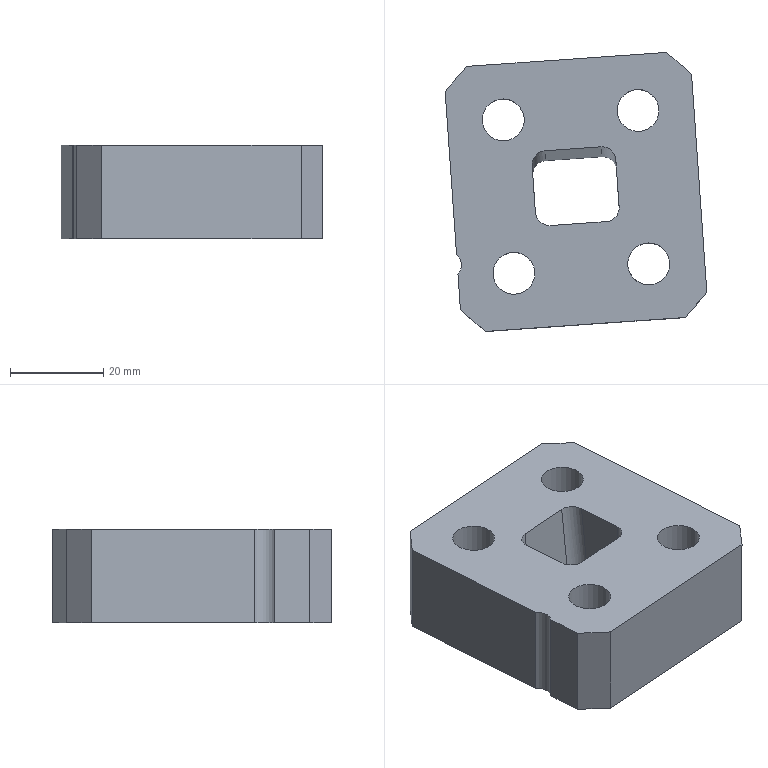Part | STEP file | 车灯-后视镜_id94_x_t | 1 solid | 32 faces | box 56.149 x 59.861 x 20 mm | volume 45570 mm3 | plane 19 | cylinder 13 | commonest cylinder face diameters 6 x5 9 x4 14 x4
STEP:
#1=CARTESIAN_POINT('',(-19.757,-26.993,-160.5));
#2=VERTEX_POINT('',#1);
#3=CARTESIAN_POINT('',(-19.757,-26.993,-140.5));
#4=VERTEX_POINT('',#3);
#5=CARTESIAN_POINT('',(-19.757,-26.993,60.));
#6=DIRECTION('',(0.,0.,1.));
#7=VECTOR('',#6,1.);
#8=LINE('',#5,#7);
#9=EDGE_CURVE('',#2,#4,#8,.T.);
#10=ORIENTED_EDGE('',*,*,#9,.F.);
#11=CARTESIAN_POINT('',(-19.225,-34.604,-160.5));
#12=VERTEX_POINT('',#11);
#13=CARTESIAN_POINT('',(-19.643,-28.63,-160.5));
#14=DIRECTION('',(-0.06976,0.9976,0.));
#15=VECTOR('',#14,1.);
#16=LINE('',#13,#15);
#17=EDGE_CURVE('',#12,#2,#16,.T.);
#18=ORIENTED_EDGE('',*,*,#17,.F.);
#19=CARTESIAN_POINT('',(-19.225,-34.604,-140.5));
#20=VERTEX_POINT('',#19);
#21=CARTESIAN_POINT('',(-19.225,-34.604,-144.5));
#22=DIRECTION('',(0.,0.,-1.));
#23=VECTOR('',#22,1.);
#24=LINE('',#21,#23);
#25=EDGE_CURVE('',#20,#12,#24,.T.);
#26=ORIENTED_EDGE('',*,*,#25,.F.);
#27=CARTESIAN_POINT('',(-19.643,-28.63,-140.5));
#28=DIRECTION('',(0.06976,-0.9976,0.));
#29=VECTOR('',#28,1.);
#30=LINE('',#27,#29);
#31=EDGE_CURVE('',#4,#20,#30,.T.);
#32=ORIENTED_EDGE('',*,*,#31,.F.);
#33=EDGE_LOOP('',(#10,#18,#26,#32));
#34=FACE_OUTER_BOUND('',#33,.T.);
#35=CARTESIAN_POINT('',(-19.643,-28.63,-138.5));
#36=DIRECTION('',(-0.9976,-0.06976,0.));
#37=DIRECTION('',(0.,0.,-1.));
#38=AXIS2_PLACEMENT_3D('',#35,#36,#37);
#39=PLANE('',#38);
#40=ADVANCED_FACE('',(#34),#39,.T.);
#41=CARTESIAN_POINT('',(-20.056,-22.715,-160.5));
#42=VERTEX_POINT('',#41);
#43=CARTESIAN_POINT('',(-22.,-25.,-160.5));
#44=DIRECTION('',(0.,0.,-1.));
#45=DIRECTION('',(0.,1.,0.));
#46=AXIS2_PLACEMENT_3D('',#43,#44,#45);
#47=CIRCLE('',#46,3.);
#48=EDGE_CURVE('',#42,#2,#47,.T.);
#49=ORIENTED_EDGE('',*,*,#48,.F.);
#50=CARTESIAN_POINT('',(-22.504,12.282,-160.5));
#51=VERTEX_POINT('',#50);
#52=CARTESIAN_POINT('',(-19.643,-28.63,-160.5));
#53=DIRECTION('',(-0.06976,0.9976,0.));
#54=VECTOR('',#53,1.);
#55=LINE('',#52,#54);
#56=EDGE_CURVE('',#42,#51,#55,.T.);
#57=ORIENTED_EDGE('',*,*,#56,.T.);
#58=CARTESIAN_POINT('',(-17.865,17.618,-160.5));
#59=VERTEX_POINT('',#58);
#60=CARTESIAN_POINT('',(-22.504,12.282,-160.5));
#61=DIRECTION('',(-0.6561,-0.7547,0.));
#62=VECTOR('',#61,1.);
#63=LINE('',#60,#62);
#64=EDGE_CURVE('',#59,#51,#63,.T.);
#65=ORIENTED_EDGE('',*,*,#64,.F.);
#66=CARTESIAN_POINT('',(25.031,20.618,-160.5));
#67=VERTEX_POINT('',#66);
#68=CARTESIAN_POINT('',(2.662,19.054,-160.5));
#69=DIRECTION('',(0.9976,0.06976,0.));
#70=VECTOR('',#69,1.);
#71=LINE('',#68,#70);
#72=EDGE_CURVE('',#59,#67,#71,.T.);
#73=ORIENTED_EDGE('',*,*,#72,.T.);
#74=CARTESIAN_POINT('',(30.367,15.979,-160.5));
#75=VERTEX_POINT('',#74);
#76=CARTESIAN_POINT('',(25.031,20.618,-160.5));
#77=DIRECTION('',(-0.7547,0.6561,0.));
#78=VECTOR('',#77,1.);
#79=LINE('',#76,#78);
#80=EDGE_CURVE('',#75,#67,#79,.T.);
#81=ORIENTED_EDGE('',*,*,#80,.F.);
#82=CARTESIAN_POINT('',(33.646,-30.907,-160.5));
#83=VERTEX_POINT('',#82);
#84=CARTESIAN_POINT('',(33.228,-24.933,-160.5));
#85=DIRECTION('',(0.06976,-0.9976,0.));
#86=VECTOR('',#85,1.);
#87=LINE('',#84,#86);
#88=EDGE_CURVE('',#75,#83,#87,.T.);
#89=ORIENTED_EDGE('',*,*,#88,.T.);
#90=CARTESIAN_POINT('',(29.007,-36.243,-160.5));
#91=VERTEX_POINT('',#90);
#92=CARTESIAN_POINT('',(29.007,-36.243,-160.5));
#93=DIRECTION('',(0.6561,0.7547,0.));
#94=VECTOR('',#93,1.);
#95=LINE('',#92,#94);
#96=EDGE_CURVE('',#91,#83,#95,.T.);
#97=ORIENTED_EDGE('',*,*,#96,.F.);
#98=CARTESIAN_POINT('',(-13.889,-39.243,-160.5));
#99=VERTEX_POINT('',#98);
#100=CARTESIAN_POINT('',(6.639,-37.808,-160.5));
#101=DIRECTION('',(-0.9976,-0.06976,0.));
#102=VECTOR('',#101,1.);
#103=LINE('',#100,#102);
#104=EDGE_CURVE('',#91,#99,#103,.T.);
#105=ORIENTED_EDGE('',*,*,#104,.T.);
#106=CARTESIAN_POINT('',(-13.889,-39.243,-160.5));
#107=DIRECTION('',(0.7547,-0.6561,0.));
#108=VECTOR('',#107,1.);
#109=LINE('',#106,#108);
#110=EDGE_CURVE('',#12,#99,#109,.T.);
#111=ORIENTED_EDGE('',*,*,#110,.F.);
#112=ORIENTED_EDGE('',*,*,#17,.T.);
#113=EDGE_LOOP('',(#49,#57,#65,#73,#81,#89,#97,#105,#111,#112));
#114=FACE_BOUND('',#113,.T.);
#115=CARTESIAN_POINT('',(-9.984,-0.864,-160.5));
#116=VERTEX_POINT('',#115);
#117=CARTESIAN_POINT('',(-10.045,6.136,-160.5));
#118=DIRECTION('',(0.,0.,1.));
#119=DIRECTION('',(0.008727,-1.,0.));
#120=AXIS2_PLACEMENT_3D('',#117,#118,#119);
#121=CIRCLE('',#120,7.);
#122=EDGE_CURVE('',#116,#116,#121,.T.);
#123=ORIENTED_EDGE('',*,*,#122,.T.);
#124=EDGE_LOOP('',(#123));
#125=FACE_BOUND('',#124,.T.);
#126=CARTESIAN_POINT('',(-7.743,-19.784,-160.5));
#127=VERTEX_POINT('',#126);
#128=CARTESIAN_POINT('',(-7.743,-26.784,-160.5));
#129=DIRECTION('',(0.,0.,-1.));
#130=DIRECTION('',(0.,1.,0.));
#131=AXIS2_PLACEMENT_3D('',#128,#129,#130);
#132=CIRCLE('',#131,7.);
#133=EDGE_CURVE('',#127,#127,#132,.T.);
#134=ORIENTED_EDGE('',*,*,#133,.F.);
#135=EDGE_LOOP('',(#134));
#136=FACE_BOUND('',#135,.T.);
#137=CARTESIAN_POINT('',(18.885,15.159,-160.5));
#138=VERTEX_POINT('',#137);
#139=CARTESIAN_POINT('',(18.885,8.159,-160.5));
#140=DIRECTION('',(0.,0.,-1.));
#141=DIRECTION('',(0.,1.,0.));
#142=AXIS2_PLACEMENT_3D('',#139,#140,#141);
#143=CIRCLE('',#142,7.);
#144=EDGE_CURVE('',#138,#138,#143,.T.);
#145=ORIENTED_EDGE('',*,*,#144,.F.);
#146=EDGE_LOOP('',(#145));
#147=FACE_BOUND('',#146,.T.);
#148=CARTESIAN_POINT('',(21.187,-17.761,-160.5));
#149=VERTEX_POINT('',#148);
#150=CARTESIAN_POINT('',(21.187,-24.761,-160.5));
#151=DIRECTION('',(0.,0.,1.));
#152=DIRECTION('',(0.,1.,0.));
#153=AXIS2_PLACEMENT_3D('',#150,#151,#152);
#154=CIRCLE('',#153,7.);
#155=EDGE_CURVE('',#149,#149,#154,.T.);
#156=ORIENTED_EDGE('',*,*,#155,.T.);
#157=EDGE_LOOP('',(#156));
#158=FACE_BOUND('',#157,.T.);
#159=CARTESIAN_POINT('',(-3.697,-5.793,-160.5));
#160=VERTEX_POINT('',#159);
#161=CARTESIAN_POINT('',(-0.9148,-2.575,-160.5));
#162=VERTEX_POINT('',#161);
#163=CARTESIAN_POINT('',(-0.7043,-5.584,-160.5));
#164=DIRECTION('',(0.,0.,-1.));
#165=DIRECTION('',(-0.06976,0.9976,0.));
#166=AXIS2_PLACEMENT_3D('',#163,#164,#165);
#167=ELLIPSE('',#166,3.017,3.);
#168=EDGE_CURVE('',#160,#162,#167,.T.);
#169=ORIENTED_EDGE('',*,*,#168,.F.);
#170=CARTESIAN_POINT('',(-2.996,-15.824,-160.5));
#171=VERTEX_POINT('',#170);
#172=CARTESIAN_POINT('',(-2.185,-27.409,-160.5));
#173=DIRECTION('',(0.06976,-0.9976,0.));
#174=VECTOR('',#173,1.);
#175=LINE('',#172,#174);
#176=EDGE_CURVE('',#160,#171,#175,.T.);
#177=ORIENTED_EDGE('',*,*,#176,.T.);
#178=CARTESIAN_POINT('',(0.2075,-18.624,-160.5));
#179=VERTEX_POINT('',#178);
#180=CARTESIAN_POINT('',(-0.002931,-15.614,-160.5));
#181=DIRECTION('',(0.,0.,-1.));
#182=DIRECTION('',(-0.06976,0.9976,0.));
#183=AXIS2_PLACEMENT_3D('',#180,#181,#182);
#184=ELLIPSE('',#183,3.017,3.);
#185=EDGE_CURVE('',#179,#171,#184,.T.);
#186=ORIENTED_EDGE('',*,*,#185,.F.);
#187=CARTESIAN_POINT('',(12.178,-17.786,-160.5));
#188=VERTEX_POINT('',#187);
#189=CARTESIAN_POINT('',(5.272,-18.269,-160.5));
#190=DIRECTION('',(-0.9976,-0.06976,0.));
#191=VECTOR('',#190,1.);
#192=LINE('',#189,#191);
#193=EDGE_CURVE('',#188,#179,#192,.T.);
#194=ORIENTED_EDGE('',*,*,#193,.F.);
#195=CARTESIAN_POINT('',(14.961,-14.568,-160.5));
#196=VERTEX_POINT('',#195);
#197=CARTESIAN_POINT('',(11.968,-14.777,-160.5));
#198=DIRECTION('',(0.,0.,-1.));
#199=DIRECTION('',(0.06976,-0.9976,0.));
#200=AXIS2_PLACEMENT_3D('',#197,#198,#199);
#201=ELLIPSE('',#200,3.017,3.);
#202=EDGE_CURVE('',#196,#188,#201,.T.);
#203=ORIENTED_EDGE('',*,*,#202,.F.);
#204=CARTESIAN_POINT('',(14.259,-4.537,-160.5));
#205=VERTEX_POINT('',#204);
#206=CARTESIAN_POINT('',(15.771,-26.154,-160.5));
#207=DIRECTION('',(0.06976,-0.9976,0.));
#208=VECTOR('',#207,1.);
#209=LINE('',#206,#208);
#210=EDGE_CURVE('',#205,#196,#209,.T.);
#211=ORIENTED_EDGE('',*,*,#210,.F.);
#212=CARTESIAN_POINT('',(11.056,-1.738,-160.5));
#213=VERTEX_POINT('',#212);
#214=CARTESIAN_POINT('',(11.266,-4.747,-160.5));
#215=DIRECTION('',(0.,0.,-1.));
#216=DIRECTION('',(-0.06976,0.9976,0.));
#217=AXIS2_PLACEMENT_3D('',#214,#215,#216);
#218=ELLIPSE('',#217,3.017,3.);
#219=EDGE_CURVE('',#213,#205,#218,.T.);
#220=ORIENTED_EDGE('',*,*,#219,.F.);
#221=CARTESIAN_POINT('',(4.15,-2.22,-160.5));
#222=DIRECTION('',(0.9976,0.06976,0.));
#223=VECTOR('',#222,1.);
#224=LINE('',#221,#223);
#225=EDGE_CURVE('',#162,#213,#224,.T.);
#226=ORIENTED_EDGE('',*,*,#225,.F.);
#227=EDGE_LOOP('',(#169,#177,#186,#194,#203,#211,#220,#226));
#228=FACE_BOUND('',#227,.T.);
#229=CARTESIAN_POINT('',(5.872,-26.846,-160.5));
#230=DIRECTION('',(0.,0.,-1.));
#231=DIRECTION('',(-0.06976,0.9976,0.));
#232=AXIS2_PLACEMENT_3D('',#229,#230,#231);
#233=PLANE('',#232);
#234=ADVANCED_FACE('',(#114,#125,#136,#147,#158,#228),#233,.T.);
#235=CARTESIAN_POINT('',(-20.056,-22.715,-140.5));
#236=VERTEX_POINT('',#235);
#237=CARTESIAN_POINT('',(-22.,-25.,-140.5));
#238=DIRECTION('',(0.,0.,1.));
#239=DIRECTION('',(0.,-1.,0.));
#240=AXIS2_PLACEMENT_3D('',#237,#238,#239);
#241=CIRCLE('',#240,3.);
#242=EDGE_CURVE('',#4,#236,#241,.T.);
#243=ORIENTED_EDGE('',*,*,#242,.F.);
#244=ORIENTED_EDGE('',*,*,#31,.T.);
#245=CARTESIAN_POINT('',(-13.889,-39.243,-140.5));
#246=VERTEX_POINT('',#245);
#247=CARTESIAN_POINT('',(-13.889,-39.243,-140.5));
#248=DIRECTION('',(-0.7547,0.6561,0.));
#249=VECTOR('',#248,1.);
#250=LINE('',#247,#249);
#251=EDGE_CURVE('',#246,#20,#250,.T.);
#252=ORIENTED_EDGE('',*,*,#251,.F.);
#253=CARTESIAN_POINT('',(29.007,-36.243,-140.5));
#254=VERTEX_POINT('',#253);
#255=CARTESIAN_POINT('',(6.639,-37.808,-140.5));
#256=DIRECTION('',(0.9976,0.06976,0.));
#257=VECTOR('',#256,1.);
#258=LINE('',#255,#257);
#259=EDGE_CURVE('',#246,#254,#258,.T.);
#260=ORIENTED_EDGE('',*,*,#259,.T.);
#261=CARTESIAN_POINT('',(33.646,-30.907,-140.5));
#262=VERTEX_POINT('',#261);
#263=CARTESIAN_POINT('',(29.007,-36.243,-140.5));
#264=DIRECTION('',(-0.6561,-0.7547,0.));
#265=VECTOR('',#264,1.);
#266=LINE('',#263,#265);
#267=EDGE_CURVE('',#262,#254,#266,.T.);
#268=ORIENTED_EDGE('',*,*,#267,.F.);
#269=CARTESIAN_POINT('',(30.367,15.979,-140.5));
#270=VERTEX_POINT('',#269);
#271=CARTESIAN_POINT('',(33.228,-24.933,-140.5));
#272=DIRECTION('',(-0.06976,0.9976,0.));
#273=VECTOR('',#272,1.);
#274=LINE('',#271,#273);
#275=EDGE_CURVE('',#262,#270,#274,.T.);
#276=ORIENTED_EDGE('',*,*,#275,.T.);
#277=CARTESIAN_POINT('',(25.031,20.618,-140.5));
#278=VERTEX_POINT('',#277);
#279=CARTESIAN_POINT('',(25.031,20.618,-140.5));
#280=DIRECTION('',(0.7547,-0.6561,0.));
#281=VECTOR('',#280,1.);
#282=LINE('',#279,#281);
#283=EDGE_CURVE('',#278,#270,#282,.T.);
#284=ORIENTED_EDGE('',*,*,#283,.F.);
#285=CARTESIAN_POINT('',(-17.865,17.618,-140.5));
#286=VERTEX_POINT('',#285);
#287=CARTESIAN_POINT('',(2.662,19.054,-140.5));
#288=DIRECTION('',(-0.9976,-0.06976,0.));
#289=VECTOR('',#288,1.);
#290=LINE('',#287,#289);
#291=EDGE_CURVE('',#278,#286,#290,.T.);
#292=ORIENTED_EDGE('',*,*,#291,.T.);
#293=CARTESIAN_POINT('',(-22.504,12.282,-140.5));
#294=VERTEX_POINT('',#293);
#295=CARTESIAN_POINT('',(-22.504,12.282,-140.5));
#296=DIRECTION('',(0.6561,0.7547,0.));
#297=VECTOR('',#296,1.);
#298=LINE('',#295,#297);
#299=EDGE_CURVE('',#294,#286,#298,.T.);
#300=ORIENTED_EDGE('',*,*,#299,.F.);
#301=CARTESIAN_POINT('',(-19.643,-28.63,-140.5));
#302=DIRECTION('',(0.06976,-0.9976,0.));
#303=VECTOR('',#302,1.);
#304=LINE('',#301,#303);
#305=EDGE_CURVE('',#294,#236,#304,.T.);
#306=ORIENTED_EDGE('',*,*,#305,.T.);
#307=EDGE_LOOP('',(#243,#244,#252,#260,#268,#276,#284,#292,#300,#306));
#308=FACE_BOUND('',#307,.T.);
#309=CARTESIAN_POINT('',(-10.084,10.636,-140.5));
#310=VERTEX_POINT('',#309);
#311=CARTESIAN_POINT('',(-10.045,6.136,-140.5));
#312=DIRECTION('',(0.,0.,-1.));
#313=DIRECTION('',(-0.008727,1.,0.));
#314=AXIS2_PLACEMENT_3D('',#311,#312,#313);
#315=CIRCLE('',#314,4.5);
#316=EDGE_CURVE('',#310,#310,#315,.T.);
#317=ORIENTED_EDGE('',*,*,#316,.T.);
#318=EDGE_LOOP('',(#317));
#319=FACE_BOUND('',#318,.T.);
#320=CARTESIAN_POINT('',(-7.743,-31.284,-140.5));
#321=VERTEX_POINT('',#320);
#322=CARTESIAN_POINT('',(-7.743,-26.784,-140.5));
#323=DIRECTION('',(0.,0.,1.));
#324=DIRECTION('',(0.,-1.,0.));
#325=AXIS2_PLACEMENT_3D('',#322,#323,#324);
#326=CIRCLE('',#325,4.5);
#327=EDGE_CURVE('',#321,#321,#326,.T.);
#328=ORIENTED_EDGE('',*,*,#327,.F.);
#329=EDGE_LOOP('',(#328));
#330=FACE_BOUND('',#329,.T.);
#331=CARTESIAN_POINT('',(18.885,3.659,-140.5));
#332=VERTEX_POINT('',#331);
#333=CARTESIAN_POINT('',(18.885,8.159,-140.5));
#334=DIRECTION('',(0.,0.,1.));
#335=DIRECTION('',(0.,-1.,0.));
#336=AXIS2_PLACEMENT_3D('',#333,#334,#335);
#337=CIRCLE('',#336,4.5);
#338=EDGE_CURVE('',#332,#332,#337,.T.);
#339=ORIENTED_EDGE('',*,*,#338,.F.);
#340=EDGE_LOOP('',(#339));
#341=FACE_BOUND('',#340,.T.);
#342=CARTESIAN_POINT('',(21.187,-29.261,-140.5));
#343=VERTEX_POINT('',#342);
#344=CARTESIAN_POINT('',(21.187,-24.761,-140.5));
#345=DIRECTION('',(0.,0.,-1.));
#346=DIRECTION('',(0.,-1.,0.));
#347=AXIS2_PLACEMENT_3D('',#344,#345,#346);
#348=CIRCLE('',#347,4.5);
#349=EDGE_CURVE('',#343,#343,#348,.T.);
#350=ORIENTED_EDGE('',*,*,#349,.T.);
#351=EDGE_LOOP('',(#350));
#352=FACE_BOUND('',#351,.T.);
#353=CARTESIAN_POINT('',(-3.142,-13.727,-140.5));
#354=VERTEX_POINT('',#353);
#355=CARTESIAN_POINT('',(0.06086,-16.527,-140.5));
#356=VERTEX_POINT('',#355);
#357=CARTESIAN_POINT('',(-0.1496,-13.517,-140.5));
#358=DIRECTION('',(0.,0.,1.));
#359=DIRECTION('',(-0.06976,0.9976,0.));
#360=AXIS2_PLACEMENT_3D('',#357,#358,#359);
#361=ELLIPSE('',#360,3.017,3.);
#362=EDGE_CURVE('',#354,#356,#361,.T.);
#363=ORIENTED_EDGE('',*,*,#362,.F.);
#364=CARTESIAN_POINT('',(-3.844,-3.696,-140.5));
#365=VERTEX_POINT('',#364);
#366=CARTESIAN_POINT('',(-2.185,-27.409,-140.5));
#367=DIRECTION('',(-0.06976,0.9976,0.));
#368=VECTOR('',#367,1.);
#369=LINE('',#366,#368);
#370=EDGE_CURVE('',#354,#365,#369,.T.);
#371=ORIENTED_EDGE('',*,*,#370,.T.);
#372=CARTESIAN_POINT('',(-1.061,-0.4776,-140.5));
#373=VERTEX_POINT('',#372);
#374=CARTESIAN_POINT('',(-0.851,-3.487,-140.5));
#375=DIRECTION('',(0.,0.,1.));
#376=DIRECTION('',(-0.06976,0.9976,0.));
#377=AXIS2_PLACEMENT_3D('',#374,#375,#376);
#378=ELLIPSE('',#377,3.017,3.);
#379=EDGE_CURVE('',#373,#365,#378,.T.);
#380=ORIENTED_EDGE('',*,*,#379,.F.);
#381=CARTESIAN_POINT('',(10.909,0.3594,-140.5));
#382=VERTEX_POINT('',#381);
#383=CARTESIAN_POINT('',(4.003,-0.1235,-140.5));
#384=DIRECTION('',(-0.9976,-0.06976,0.));
#385=VECTOR('',#384,1.);
#386=LINE('',#383,#385);
#387=EDGE_CURVE('',#382,#373,#386,.T.);
#388=ORIENTED_EDGE('',*,*,#387,.F.);
#389=CARTESIAN_POINT('',(14.112,-2.44,-140.5));
#390=VERTEX_POINT('',#389);
#391=CARTESIAN_POINT('',(11.12,-2.65,-140.5));
#392=DIRECTION('',(0.,0.,1.));
#393=DIRECTION('',(-0.06976,0.9976,0.));
#394=AXIS2_PLACEMENT_3D('',#391,#392,#393);
#395=ELLIPSE('',#394,3.017,3.);
#396=EDGE_CURVE('',#390,#382,#395,.T.);
#397=ORIENTED_EDGE('',*,*,#396,.F.);
#398=CARTESIAN_POINT('',(14.814,-12.471,-140.5));
#399=VERTEX_POINT('',#398);
#400=CARTESIAN_POINT('',(15.771,-26.154,-140.5));
#401=DIRECTION('',(-0.06976,0.9976,0.));
#402=VECTOR('',#401,1.);
#403=LINE('',#400,#402);
#404=EDGE_CURVE('',#399,#390,#403,.T.);
#405=ORIENTED_EDGE('',*,*,#404,.F.);
#406=CARTESIAN_POINT('',(12.032,-15.689,-140.5));
#407=VERTEX_POINT('',#406);
#408=CARTESIAN_POINT('',(11.821,-12.68,-140.5));
#409=DIRECTION('',(0.,0.,1.));
#410=DIRECTION('',(0.06976,-0.9976,0.));
#411=AXIS2_PLACEMENT_3D('',#408,#409,#410);
#412=ELLIPSE('',#411,3.017,3.);
#413=EDGE_CURVE('',#407,#399,#412,.T.);
#414=ORIENTED_EDGE('',*,*,#413,.F.);
#415=CARTESIAN_POINT('',(5.126,-16.172,-140.5));
#416=DIRECTION('',(0.9976,0.06976,0.));
#417=VECTOR('',#416,1.);
#418=LINE('',#415,#417);
#419=EDGE_CURVE('',#356,#407,#418,.T.);
#420=ORIENTED_EDGE('',*,*,#419,.F.);
#421=EDGE_LOOP('',(#363,#371,#380,#388,#397,#405,#414,#420));
#422=FACE_BOUND('',#421,.T.);
#423=CARTESIAN_POINT('',(5.872,-26.846,-140.5));
#424=DIRECTION('',(0.,0.,1.));
#425=DIRECTION('',(0.06976,-0.9976,0.));
#426=AXIS2_PLACEMENT_3D('',#423,#424,#425);
#427=PLANE('',#426);
#428=ADVANCED_FACE('',(#308,#319,#330,#341,#352,#422),#427,.T.);
#429=ORIENTED_EDGE('',*,*,#275,.F.);
#430=CARTESIAN_POINT('',(33.646,-30.907,-144.5));
#431=DIRECTION('',(0.,0.,1.));
#432=VECTOR('',#431,1.);
#433=LINE('',#430,#432);
#434=EDGE_CURVE('',#83,#262,#433,.T.);
#435=ORIENTED_EDGE('',*,*,#434,.F.);
#436=ORIENTED_EDGE('',*,*,#88,.F.);
#437=CARTESIAN_POINT('',(30.367,15.979,-138.5));
#438=DIRECTION('',(0.,0.,-1.));
#439=VECTOR('',#438,1.);
#440=LINE('',#437,#439);
#441=EDGE_CURVE('',#270,#75,#440,.T.);
#442=ORIENTED_EDGE('',*,*,#441,.F.);
#443=EDGE_LOOP('',(#429,#435,#436,#442));
#444=FACE_OUTER_BOUND('',#443,.T.);
#445=CARTESIAN_POINT('',(33.228,-24.933,-138.5));
#446=DIRECTION('',(0.9976,0.06976,0.));
#447=DIRECTION('',(0.,0.,1.));
#448=AXIS2_PLACEMENT_3D('',#445,#446,#447);
#449=PLANE('',#448);
#450=ADVANCED_FACE('',(#444),#449,.T.);
#451=CARTESIAN_POINT('',(-20.056,-22.715,60.));
#452=DIRECTION('',(0.,0.,-1.));
#453=VECTOR('',#452,1.);
#454=LINE('',#451,#453);
#455=EDGE_CURVE('',#236,#42,#454,.T.);
#456=ORIENTED_EDGE('',*,*,#455,.F.);
#457=ORIENTED_EDGE('',*,*,#305,.F.);
#458=CARTESIAN_POINT('',(-22.504,12.282,-138.5));
#459=DIRECTION('',(0.,0.,1.));
#460=VECTOR('',#459,1.);
#461=LINE('',#458,#460);
#462=EDGE_CURVE('',#51,#294,#461,.T.);
#463=ORIENTED_EDGE('',*,*,#462,.F.);
#464=ORIENTED_EDGE('',*,*,#56,.F.);
#465=EDGE_LOOP('',(#456,#457,#463,#464));
#466=FACE_OUTER_BOUND('',#465,.T.);
#467=CARTESIAN_POINT('',(-19.643,-28.63,-138.5));
#468=DIRECTION('',(-0.9976,-0.06976,0.));
#469=DIRECTION('',(0.,0.,-1.));
#470=AXIS2_PLACEMENT_3D('',#467,#468,#469);
#471=PLANE('',#470);
#472=ADVANCED_FACE('',(#466),#471,.T.);
#473=ORIENTED_EDGE('',*,*,#291,.F.);
#474=CARTESIAN_POINT('',(25.031,20.618,-138.5));
#475=DIRECTION('',(0.,0.,1.));
#476=VECTOR('',#475,1.);
#477=LINE('',#474,#476);
#478=EDGE_CURVE('',#67,#278,#477,.T.);
#479=ORIENTED_EDGE('',*,*,#478,.F.);
#480=ORIENTED_EDGE('',*,*,#72,.F.);
#481=CARTESIAN_POINT('',(-17.865,17.618,-138.5));
#482=DIRECTION('',(0.,0.,-1.));
#483=VECTOR('',#482,1.);
#484=LINE('',#481,#483);
#485=EDGE_CURVE('',#286,#59,#484,.T.);
#486=ORIENTED_EDGE('',*,*,#485,.F.);
#487=EDGE_LOOP('',(#473,#479,#480,#486));
#488=FACE_OUTER_BOUND('',#487,.T.);
#489=CARTESIAN_POINT('',(2.662,19.054,-138.5));
#490=DIRECTION('',(-0.06976,0.9976,0.));
#491=DIRECTION('',(0.,0.,1.));
#492=AXIS2_PLACEMENT_3D('',#489,#490,#491);
#493=PLANE('',#492);
#494=ADVANCED_FACE('',(#488),#493,.T.);
#495=CARTESIAN_POINT('',(-10.084,10.636,-152.));
#496=VERTEX_POINT('',#495);
#497=CARTESIAN_POINT('',(-10.045,6.136,-152.));
#498=DIRECTION('',(0.,0.,-1.));
#499=DIRECTION('',(-0.008727,1.,0.));
#500=AXIS2_PLACEMENT_3D('',#497,#498,#499);
#501=CIRCLE('',#500,4.5);
#502=EDGE_CURVE('',#496,#496,#501,.T.);
#503=ORIENTED_EDGE('',*,*,#502,.T.);
#504=EDGE_LOOP('',(#503));
#505=FACE_BOUND('',#504,.T.);
#506=ORIENTED_EDGE('',*,*,#316,.F.);
#507=EDGE_LOOP('',(#506));
#508=FACE_BOUND('',#507,.T.);
#509=CARTESIAN_POINT('',(-10.045,6.136,-140.5));
#510=DIRECTION('',(0.,0.,-1.));
#511=DIRECTION('',(0.06976,-0.9976,0.));
#512=AXIS2_PLACEMENT_3D('',#509,#510,#511);
#513=CYLINDRICAL_SURFACE('',#512,4.5);
#514=ADVANCED_FACE('',(#505,#508),#513,.F.);
#515=ORIENTED_EDGE('',*,*,#502,.F.);
#516=EDGE_LOOP('',(#515));
#517=FACE_BOUND('',#516,.T.);
#518=CARTESIAN_POINT('',(-10.106,13.135,-152.));
#519=VERTEX_POINT('',#518);
#520=CARTESIAN_POINT('',(-10.045,6.136,-152.));
#521=DIRECTION('',(0.,0.,-1.));
#522=DIRECTION('',(-0.008727,1.,0.));
#523=AXIS2_PLACEMENT_3D('',#520,#521,#522);
#524=CIRCLE('',#523,7.);
#525=EDGE_CURVE('',#519,#519,#524,.T.);
#526=ORIENTED_EDGE('',*,*,#525,.T.);
#527=EDGE_LOOP('',(#526));
#528=FACE_BOUND('',#527,.T.);
#529=CARTESIAN_POINT('',(-10.045,6.136,-152.));
#530=DIRECTION('',(0.,0.,1.));
#531=DIRECTION('',(-0.06976,0.9976,0.));
#532=AXIS2_PLACEMENT_3D('',#529,#530,#531);
#533=PLANE('',#532);
#534=ADVANCED_FACE('',(#517,#528),#533,.F.);
#535=ORIENTED_EDGE('',*,*,#525,.F.);
#536=EDGE_LOOP('',(#535));
#537=FACE_BOUND('',#536,.T.);
#538=ORIENTED_EDGE('',*,*,#122,.F.);
#539=EDGE_LOOP('',(#538));
#540=FACE_BOUND('',#539,.T.);
#541=CARTESIAN_POINT('',(-10.045,6.136,-150.5));
#542=DIRECTION('',(0.,0.,1.));
#543=DIRECTION('',(-0.06976,0.9976,0.));
#544=AXIS2_PLACEMENT_3D('',#541,#542,#543);
#545=CYLINDRICAL_SURFACE('',#544,7.);
#546=ADVANCED_FACE('',(#537,#540),#545,.F.);
#547=CARTESIAN_POINT('',(-7.782,-22.284,-152.));
#548=VERTEX_POINT('',#547);
#549=CARTESIAN_POINT('',(-7.743,-26.784,-152.));
#550=DIRECTION('',(0.,0.,1.));
#551=DIRECTION('',(-0.008727,1.,0.));
#552=AXIS2_PLACEMENT_3D('',#549,#550,#551);
#553=CIRCLE('',#552,4.5);
#554=EDGE_CURVE('',#548,#548,#553,.T.);
#555=ORIENTED_EDGE('',*,*,#554,.F.);
#556=EDGE_LOOP('',(#555));
#557=FACE_BOUND('',#556,.T.);
#558=ORIENTED_EDGE('',*,*,#327,.T.);
#559=EDGE_LOOP('',(#558));
#560=FACE_BOUND('',#559,.T.);
#561=CARTESIAN_POINT('',(-7.743,-26.784,-140.5));
#562=DIRECTION('',(0.,0.,-1.));
#563=DIRECTION('',(-0.06976,0.9976,0.));
#564=AXIS2_PLACEMENT_3D('',#561,#562,#563);
#565=CYLINDRICAL_SURFACE('',#564,4.5);
#566=ADVANCED_FACE('',(#557,#560),#565,.F.);
#567=ORIENTED_EDGE('',*,*,#554,.T.);
#568=EDGE_LOOP('',(#567));
#569=FACE_BOUND('',#568,.T.);
#570=CARTESIAN_POINT('',(-7.804,-19.784,-152.));
#571=VERTEX_POINT('',#570);
#572=CARTESIAN_POINT('',(-7.743,-26.784,-152.));
#573=DIRECTION('',(0.,0.,1.));
#574=DIRECTION('',(-0.008727,1.,0.));
#575=AXIS2_PLACEMENT_3D('',#572,#573,#574);
#576=CIRCLE('',#575,7.);
#577=EDGE_CURVE('',#571,#571,#576,.T.);
#578=ORIENTED_EDGE('',*,*,#577,.F.);
#579=EDGE_LOOP('',(#578));
#580=FACE_BOUND('',#579,.T.);
#581=CARTESIAN_POINT('',(-7.743,-26.784,-152.));
#582=DIRECTION('',(0.,0.,1.));
#583=DIRECTION('',(0.06976,-0.9976,0.));
#584=AXIS2_PLACEMENT_3D('',#581,#582,#583);
#585=PLANE('',#584);
#586=ADVANCED_FACE('',(#569,#580),#585,.F.);
#587=ORIENTED_EDGE('',*,*,#577,.T.);
#588=EDGE_LOOP('',(#587));
#589=FACE_BOUND('',#588,.T.);
#590=ORIENTED_EDGE('',*,*,#133,.T.);
#591=EDGE_LOOP('',(#590));
#592=FACE_BOUND('',#591,.T.);
#593=CARTESIAN_POINT('',(-7.743,-26.784,-150.5));
#594=DIRECTION('',(0.,0.,1.));
#595=DIRECTION('',(0.06976,-0.9976,0.));
#596=AXIS2_PLACEMENT_3D('',#593,#594,#595);
#597=CYLINDRICAL_SURFACE('',#596,7.);
#598=ADVANCED_FACE('',(#589,#592),#597,.F.);
#599=CARTESIAN_POINT('',(18.845,12.659,-152.));
#600=VERTEX_POINT('',#599);
#601=CARTESIAN_POINT('',(18.885,8.159,-152.));
#602=DIRECTION('',(0.,0.,1.));
#603=DIRECTION('',(-0.008727,1.,0.));
#604=AXIS2_PLACEMENT_3D('',#601,#602,#603);
#605=CIRCLE('',#604,4.5);
#606=EDGE_CURVE('',#600,#600,#605,.T.);
#607=ORIENTED_EDGE('',*,*,#606,.F.);
#608=EDGE_LOOP('',(#607));
#609=FACE_BOUND('',#608,.T.);
#610=ORIENTED_EDGE('',*,*,#338,.T.);
#611=EDGE_LOOP('',(#610));
#612=FACE_BOUND('',#611,.T.);
#613=CARTESIAN_POINT('',(18.885,8.159,-140.5));
#614=DIRECTION('',(0.,0.,-1.));
#615=DIRECTION('',(0.06976,-0.9976,0.));
#616=AXIS2_PLACEMENT_3D('',#613,#614,#615);
#617=CYLINDRICAL_SURFACE('',#616,4.5);
#618=ADVANCED_FACE('',(#609,#612),#617,.F.);
#619=ORIENTED_EDGE('',*,*,#606,.T.);
#620=EDGE_LOOP('',(#619));
#621=FACE_BOUND('',#620,.T.);
#622=CARTESIAN_POINT('',(18.824,15.158,-152.));
#623=VERTEX_POINT('',#622);
#624=CARTESIAN_POINT('',(18.885,8.159,-152.));
#625=DIRECTION('',(0.,0.,1.));
#626=DIRECTION('',(-0.008727,1.,0.));
#627=AXIS2_PLACEMENT_3D('',#624,#625,#626);
#628=CIRCLE('',#627,7.);
#629=EDGE_CURVE('',#623,#623,#628,.T.);
#630=ORIENTED_EDGE('',*,*,#629,.F.);
#631=EDGE_LOOP('',(#630));
#632=FACE_BOUND('',#631,.T.);
#633=CARTESIAN_POINT('',(18.885,8.159,-152.));
#634=DIRECTION('',(0.,0.,1.));
#635=DIRECTION('',(-0.06976,0.9976,0.));
#636=AXIS2_PLACEMENT_3D('',#633,#634,#635);
#637=PLANE('',#636);
#638=ADVANCED_FACE('',(#621,#632),#637,.F.);
#639=ORIENTED_EDGE('',*,*,#629,.T.);
#640=EDGE_LOOP('',(#639));
#641=FACE_BOUND('',#640,.T.);
#642=ORIENTED_EDGE('',*,*,#144,.T.);
#643=EDGE_LOOP('',(#642));
#644=FACE_BOUND('',#643,.T.);
#645=CARTESIAN_POINT('',(18.885,8.159,-150.5));
#646=DIRECTION('',(0.,0.,1.));
#647=DIRECTION('',(-0.06976,0.9976,0.));
#648=AXIS2_PLACEMENT_3D('',#645,#646,#647);
#649=CYLINDRICAL_SURFACE('',#648,7.);
#650=ADVANCED_FACE('',(#641,#644),#649,.F.);
#651=CARTESIAN_POINT('',(21.147,-20.261,-152.));
#652=VERTEX_POINT('',#651);
#653=CARTESIAN_POINT('',(21.187,-24.761,-152.));
#654=DIRECTION('',(0.,0.,-1.));
#655=DIRECTION('',(-0.008727,1.,0.));
#656=AXIS2_PLACEMENT_3D('',#653,#654,#655);
#657=CIRCLE('',#656,4.5);
#658=EDGE_CURVE('',#652,#652,#657,.T.);
#659=ORIENTED_EDGE('',*,*,#658,.T.);
#660=EDGE_LOOP('',(#659));
#661=FACE_BOUND('',#660,.T.);
#662=ORIENTED_EDGE('',*,*,#349,.F.);
#663=EDGE_LOOP('',(#662));
#664=FACE_BOUND('',#663,.T.);
#665=CARTESIAN_POINT('',(21.187,-24.761,-140.5));
#666=DIRECTION('',(0.,0.,-1.));
#667=DIRECTION('',(-0.06976,0.9976,0.));
#668=AXIS2_PLACEMENT_3D('',#665,#666,#667);
#669=CYLINDRICAL_SURFACE('',#668,4.5);
#670=ADVANCED_FACE('',(#661,#664),#669,.F.);
#671=ORIENTED_EDGE('',*,*,#658,.F.);
#672=EDGE_LOOP('',(#671));
#673=FACE_BOUND('',#672,.T.);
#674=CARTESIAN_POINT('',(21.126,-17.761,-152.));
#675=VERTEX_POINT('',#674);
#676=CARTESIAN_POINT('',(21.187,-24.761,-152.));
#677=DIRECTION('',(0.,0.,-1.));
#678=DIRECTION('',(-0.008727,1.,0.));
#679=AXIS2_PLACEMENT_3D('',#676,#677,#678);
#680=CIRCLE('',#679,7.);
#681=EDGE_CURVE('',#675,#675,#680,.T.);
#682=ORIENTED_EDGE('',*,*,#681,.T.);
#683=EDGE_LOOP('',(#682));
#684=FACE_BOUND('',#683,.T.);
#685=CARTESIAN_POINT('',(21.187,-24.761,-152.));
#686=DIRECTION('',(0.,0.,1.));
#687=DIRECTION('',(0.06976,-0.9976,0.));
#688=AXIS2_PLACEMENT_3D('',#685,#686,#687);
#689=PLANE('',#688);
#690=ADVANCED_FACE('',(#673,#684),#689,.F.);
#691=ORIENTED_EDGE('',*,*,#681,.F.);
#692=EDGE_LOOP('',(#691));
#693=FACE_BOUND('',#692,.T.);
#694=ORIENTED_EDGE('',*,*,#155,.F.);
#695=EDGE_LOOP('',(#694));
#696=FACE_BOUND('',#695,.T.);
#697=CARTESIAN_POINT('',(21.187,-24.761,-150.5));
#698=DIRECTION('',(0.,0.,1.));
#699=DIRECTION('',(0.06976,-0.9976,0.));
#700=AXIS2_PLACEMENT_3D('',#697,#698,#699);
#701=CYLINDRICAL_SURFACE('',#700,7.);
#702=ADVANCED_FACE('',(#693,#696),#701,.F.);
#703=ORIENTED_EDGE('',*,*,#259,.F.);
#704=CARTESIAN_POINT('',(-13.889,-39.243,-144.5));
#705=DIRECTION('',(0.,0.,1.));
#706=VECTOR('',#705,1.);
#707=LINE('',#704,#706);
#708=EDGE_CURVE('',#99,#246,#707,.T.);
#709=ORIENTED_EDGE('',*,*,#708,.F.);
#710=ORIENTED_EDGE('',*,*,#104,.F.);
#711=CARTESIAN_POINT('',(29.007,-36.243,-144.5));
#712=DIRECTION('',(0.,0.,-1.));
#713=VECTOR('',#712,1.);
#714=LINE('',#711,#713);
#715=EDGE_CURVE('',#254,#91,#714,.T.);
#716=ORIENTED_EDGE('',*,*,#715,.F.);
#717=EDGE_LOOP('',(#703,#709,#710,#716));
#718=FACE_OUTER_BOUND('',#717,.T.);
#719=CARTESIAN_POINT('',(6.639,-37.808,-144.5));
#720=DIRECTION('',(-0.06976,0.9976,0.));
#721=DIRECTION('',(0.,0.,-1.));
#722=AXIS2_PLACEMENT_3D('',#719,#720,#721);
#723=PLANE('',#722);
#724=ADVANCED_FACE('',(#718),#723,.F.);
#725=ORIENTED_EDGE('',*,*,#267,.T.);
#726=ORIENTED_EDGE('',*,*,#715,.T.);
#727=ORIENTED_EDGE('',*,*,#96,.T.);
#728=ORIENTED_EDGE('',*,*,#434,.T.);
#729=EDGE_LOOP('',(#725,#726,#727,#728));
#730=FACE_OUTER_BOUND('',#729,.T.);
#731=CARTESIAN_POINT('',(29.007,-36.243,-144.5));
#732=DIRECTION('',(0.7547,-0.6561,0.));
#733=DIRECTION('',(0.6561,0.7547,0.));
#734=AXIS2_PLACEMENT_3D('',#731,#732,#733);
#735=PLANE('',#734);
#736=ADVANCED_FACE('',(#730),#735,.T.);
#737=ORIENTED_EDGE('',*,*,#110,.T.);
#738=ORIENTED_EDGE('',*,*,#708,.T.);
#739=ORIENTED_EDGE('',*,*,#251,.T.);
#740=ORIENTED_EDGE('',*,*,#25,.T.);
#741=EDGE_LOOP('',(#737,#738,#739,#740));
#742=FACE_OUTER_BOUND('',#741,.T.);
#743=CARTESIAN_POINT('',(-13.889,-39.243,-144.5));
#744=DIRECTION('',(-0.6561,-0.7547,0.));
#745=DIRECTION('',(0.7547,-0.6561,0.));
#746=AXIS2_PLACEMENT_3D('',#743,#744,#745);
#747=PLANE('',#746);
#748=ADVANCED_FACE('',(#742),#747,.T.);
#749=ORIENTED_EDGE('',*,*,#64,.T.);
#750=ORIENTED_EDGE('',*,*,#462,.T.);
#751=ORIENTED_EDGE('',*,*,#299,.T.);
#752=ORIENTED_EDGE('',*,*,#485,.T.);
#753=EDGE_LOOP('',(#749,#750,#751,#752));
#754=FACE_OUTER_BOUND('',#753,.T.);
#755=CARTESIAN_POINT('',(-22.504,12.282,-138.5));
#756=DIRECTION('',(0.7547,-0.6561,0.));
#757=DIRECTION('',(0.6561,0.7547,0.));
#758=AXIS2_PLACEMENT_3D('',#755,#756,#757);
#759=PLANE('',#758);
#760=ADVANCED_FACE('',(#754),#759,.F.);
#761=ORIENTED_EDGE('',*,*,#80,.T.);
#762=ORIENTED_EDGE('',*,*,#478,.T.);
#763=ORIENTED_EDGE('',*,*,#283,.T.);
#764=ORIENTED_EDGE('',*,*,#441,.T.);
#765=EDGE_LOOP('',(#761,#762,#763,#764));
#766=FACE_OUTER_BOUND('',#765,.T.);
#767=CARTESIAN_POINT('',(25.031,20.618,-138.5));
#768=DIRECTION('',(-0.6561,-0.7547,0.));
#769=DIRECTION('',(0.7547,-0.6561,0.));
#770=AXIS2_PLACEMENT_3D('',#767,#768,#769);
#771=PLANE('',#770);
#772=ADVANCED_FACE('',(#766),#771,.F.);
#773=CARTESIAN_POINT('',(-5.103,14.319,31.323));
#774=DIRECTION('',(0.007292,-0.1043,-0.9945));
#775=VECTOR('',#774,1.);
#776=LINE('',#773,#775);
#777=EDGE_CURVE('',#365,#160,#776,.T.);
#778=ORIENTED_EDGE('',*,*,#777,.F.);
#779=ORIENTED_EDGE('',*,*,#370,.F.);
#780=CARTESIAN_POINT('',(-4.588,6.949,56.696));
#781=DIRECTION('',(-0.007292,0.1043,0.9945));
#782=VECTOR('',#781,1.);
#783=LINE('',#780,#782);
#784=EDGE_CURVE('',#171,#354,#783,.T.);
#785=ORIENTED_EDGE('',*,*,#784,.F.);
#786=ORIENTED_EDGE('',*,*,#176,.F.);
#787=EDGE_LOOP('',(#778,#779,#785,#786));
#788=FACE_OUTER_BOUND('',#787,.T.);
#789=CARTESIAN_POINT('',(-4.415,4.473,65.331));
#790=DIRECTION('',(0.9976,0.06976,0.));
#791=DIRECTION('',(-0.06976,0.9976,0.000000005));
#792=AXIS2_PLACEMENT_3D('',#789,#790,#791);
#793=PLANE('',#792);
#794=ADVANCED_FACE('',(#788),#793,.T.);
#795=ORIENTED_EDGE('',*,*,#185,.T.);
#796=ORIENTED_EDGE('',*,*,#784,.T.);
#797=ORIENTED_EDGE('',*,*,#362,.T.);
#798=CARTESIAN_POINT('',(-0.09684,-14.271,-118.991));
#799=DIRECTION('',(0.007292,-0.1043,-0.9945));
#800=VECTOR('',#799,1.);
#801=LINE('',#798,#800);
#802=EDGE_CURVE('',#356,#179,#801,.T.);
#803=ORIENTED_EDGE('',*,*,#802,.T.);
#804=EDGE_LOOP('',(#795,#796,#797,#803));
#805=FACE_OUTER_BOUND('',#804,.T.);
#806=CARTESIAN_POINT('',(-1.595,7.158,56.696));
#807=DIRECTION('',(-0.007292,0.1043,0.9945));
#808=DIRECTION('',(0.,-0.9945,0.1043));
#809=AXIS2_PLACEMENT_3D('',#806,#807,#808);
#810=CYLINDRICAL_SURFACE('',#809,3.);
#811=ADVANCED_FACE('',(#805),#810,.F.);
#812=ORIENTED_EDGE('',*,*,#168,.T.);
#813=CARTESIAN_POINT('',(-2.509,20.231,57.009));
#814=DIRECTION('',(-0.007292,0.1043,0.9945));
#815=VECTOR('',#814,1.);
#816=LINE('',#813,#815);
#817=EDGE_CURVE('',#162,#373,#816,.T.);
#818=ORIENTED_EDGE('',*,*,#817,.T.);
#819=ORIENTED_EDGE('',*,*,#379,.T.);
#820=ORIENTED_EDGE('',*,*,#777,.T.);
#821=EDGE_LOOP('',(#812,#818,#819,#820));
#822=FACE_OUTER_BOUND('',#821,.T.);
#823=CARTESIAN_POINT('',(-2.35,17.948,63.933));
#824=DIRECTION('',(-0.007292,0.1043,0.9945));
#825=DIRECTION('',(0.,-0.9945,0.1043));
#826=AXIS2_PLACEMENT_3D('',#823,#824,#825);
#827=CYLINDRICAL_SURFACE('',#826,3.);
#828=ADVANCED_FACE('',(#822),#827,.F.);
#829=ORIENTED_EDGE('',*,*,#225,.T.);
#830=CARTESIAN_POINT('',(9.461,21.066,56.986));
#831=DIRECTION('',(0.007292,-0.1043,-0.9945));
#832=VECTOR('',#831,1.);
#833=LINE('',#830,#832);
#834=EDGE_CURVE('',#382,#213,#833,.T.);
#835=ORIENTED_EDGE('',*,*,#834,.F.);
#836=ORIENTED_EDGE('',*,*,#387,.T.);
#837=ORIENTED_EDGE('',*,*,#817,.F.);
#838=EDGE_LOOP('',(#829,#835,#836,#837));
#839=FACE_OUTER_BOUND('',#838,.T.);
#840=CARTESIAN_POINT('',(12.454,21.275,56.986));
#841=DIRECTION('',(-0.06937,0.9921,-0.1045));
#842=DIRECTION('',(0.,0.1048,0.9945));
#843=AXIS2_PLACEMENT_3D('',#840,#841,#842);
#844=PLANE('',#843);
#845=ADVANCED_FACE('',(#839),#844,.F.);
#846=ORIENTED_EDGE('',*,*,#219,.T.);
#847=CARTESIAN_POINT('',(12.861,15.455,30.178));
#848=DIRECTION('',(-0.007292,0.1043,0.9945));
#849=VECTOR('',#848,1.);
#850=LINE('',#847,#849);
#851=EDGE_CURVE('',#205,#390,#850,.T.);
#852=ORIENTED_EDGE('',*,*,#851,.T.);
#853=ORIENTED_EDGE('',*,*,#396,.T.);
#854=ORIENTED_EDGE('',*,*,#834,.T.);
#855=EDGE_LOOP('',(#846,#852,#853,#854));
#856=FACE_OUTER_BOUND('',#855,.T.);
#857=CARTESIAN_POINT('',(9.868,15.246,30.178));
#858=DIRECTION('',(-0.007292,0.1043,0.9945));
#859=DIRECTION('',(0.,-0.9945,0.1043));
#860=AXIS2_PLACEMENT_3D('',#857,#858,#859);
#861=CYLINDRICAL_SURFACE('',#860,3.);
#862=ADVANCED_FACE('',(#856),#861,.F.);
#863=ORIENTED_EDGE('',*,*,#193,.T.);
#864=ORIENTED_EDGE('',*,*,#802,.F.);
#865=ORIENTED_EDGE('',*,*,#419,.T.);
#866=CARTESIAN_POINT('',(10.584,5.019,57.009));
#867=DIRECTION('',(-0.007292,0.1043,0.9945));
#868=VECTOR('',#867,1.);
#869=LINE('',#866,#868);
#870=EDGE_CURVE('',#188,#407,#869,.T.);
#871=ORIENTED_EDGE('',*,*,#870,.F.);
#872=EDGE_LOOP('',(#863,#864,#865,#871));
#873=FACE_OUTER_BOUND('',#872,.T.);
#874=CARTESIAN_POINT('',(13.576,5.228,57.009));
#875=DIRECTION('',(0.06937,-0.9921,0.1045));
#876=DIRECTION('',(0.,-0.1048,-0.9945));
#877=AXIS2_PLACEMENT_3D('',#874,#875,#876);
#878=PLANE('',#877);
#879=ADVANCED_FACE('',(#873),#878,.F.);
#880=ORIENTED_EDGE('',*,*,#202,.T.);
#881=ORIENTED_EDGE('',*,*,#870,.T.);
#882=ORIENTED_EDGE('',*,*,#413,.T.);
#883=CARTESIAN_POINT('',(13.555,5.534,31.223));
#884=DIRECTION('',(0.007292,-0.1043,-0.9945));
#885=VECTOR('',#884,1.);
#886=LINE('',#883,#885);
#887=EDGE_CURVE('',#399,#196,#886,.T.);
#888=ORIENTED_EDGE('',*,*,#887,.T.);
#889=EDGE_LOOP('',(#880,#881,#882,#888));
#890=FACE_OUTER_BOUND('',#889,.T.);
#891=CARTESIAN_POINT('',(10.562,5.325,31.223));
#892=DIRECTION('',(0.007292,-0.1043,-0.9945));
#893=DIRECTION('',(0.,0.9945,-0.1043));
#894=AXIS2_PLACEMENT_3D('',#891,#892,#893);
#895=CYLINDRICAL_SURFACE('',#894,3.);
#896=ADVANCED_FACE('',(#890),#895,.F.);
#897=ORIENTED_EDGE('',*,*,#210,.T.);
#898=ORIENTED_EDGE('',*,*,#887,.F.);
#899=ORIENTED_EDGE('',*,*,#404,.T.);
#900=ORIENTED_EDGE('',*,*,#851,.F.);
#901=EDGE_LOOP('',(#897,#898,#899,#900));
#902=FACE_OUTER_BOUND('',#901,.T.);
#903=CARTESIAN_POINT('',(13.413,7.563,31.009));
#904=DIRECTION('',(0.9976,0.06976,0.));
#905=DIRECTION('',(0.,0.,-1.));
#906=AXIS2_PLACEMENT_3D('',#903,#904,#905);
#907=PLANE('',#906);
#908=ADVANCED_FACE('',(#902),#907,.F.);
#909=ORIENTED_EDGE('',*,*,#9,.T.);
#910=ORIENTED_EDGE('',*,*,#242,.T.);
#911=ORIENTED_EDGE('',*,*,#455,.T.);
#912=ORIENTED_EDGE('',*,*,#48,.T.);
#913=EDGE_LOOP('',(#909,#910,#911,#912));
#914=FACE_OUTER_BOUND('',#913,.T.);
#915=CARTESIAN_POINT('',(-22.,-25.,60.));
#916=DIRECTION('',(0.,0.,1.));
#917=DIRECTION('',(1.,0.,0.));
#918=AXIS2_PLACEMENT_3D('',#915,#916,#917);
#919=CYLINDRICAL_SURFACE('',#918,3.);
#920=ADVANCED_FACE('',(#914),#919,.F.);
#921=CLOSED_SHELL('',(#40,#234,#428,#450,#472,#494,#514,#534,#546,#566,#586,#598,#618,#638,#650,#670,#690,#702,#724,#736,#748,#760,#772,#794,#811,#828,#845,#862,#879,#896,#908,#920));
#922=MANIFOLD_SOLID_BREP('',#921);
#923=(LENGTH_UNIT()NAMED_UNIT(*)SI_UNIT(.MILLI.,.METRE.));
#924=UNCERTAINTY_MEASURE_WITH_UNIT(LENGTH_MEASURE(0.00002),#923,'','');
#925=(NAMED_UNIT(*)PLANE_ANGLE_UNIT()SI_UNIT($,.RADIAN.));
#926=PLANE_ANGLE_MEASURE_WITH_UNIT(PLANE_ANGLE_MEASURE(0.01745),#925);
#927=DIMENSIONAL_EXPONENTS(0.,0.,0.,0.,0.,0.,0.);
#928=(CONVERSION_BASED_UNIT('DEGREE',#926)NAMED_UNIT(#927)PLANE_ANGLE_UNIT());
#929=(NAMED_UNIT(*)SI_UNIT($,.STERADIAN.)SOLID_ANGLE_UNIT());
#930=(GEOMETRIC_REPRESENTATION_CONTEXT(3)GLOBAL_UNCERTAINTY_ASSIGNED_CONTEXT((#924))GLOBAL_UNIT_ASSIGNED_CONTEXT((#923,#928,#929))REPRESENTATION_CONTEXT('',''));
#931=ADVANCED_BREP_SHAPE_REPRESENTATION('',(#922),#930);